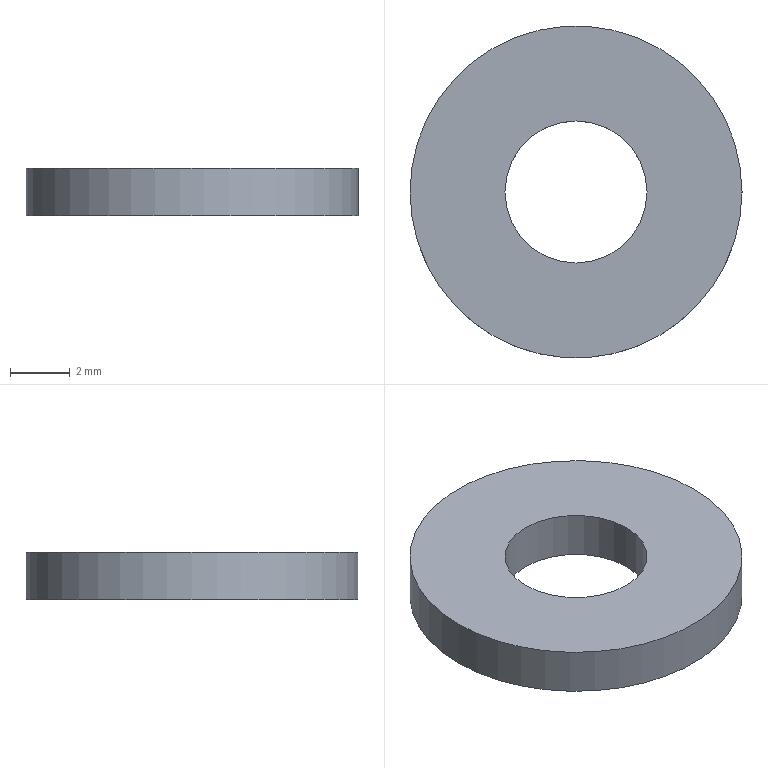Part | NX | features solid 2 | 1 solid | 4 faces | box 11.125 x 11.125 x 1.6 mm | volume 127.031 mm3 | cylinder 2 | plane 2 | commonest cylinder face diameters 4.763 x1 11.125 x1
STEP:
#1=CARTESIAN_POINT('',(5.563,0.,1.6));
#2=VERTEX_POINT('',#1);
#3=CARTESIAN_POINT('',(0.,0.,1.6));
#4=DIRECTION('',(0.,0.,1.));
#5=DIRECTION('',(1.,0.,0.));
#6=AXIS2_PLACEMENT_3D('',#3,#4,#5);
#7=CIRCLE('',#6,5.563);
#8=EDGE_CURVE('',#2,#2,#7,.T.);
#9=ORIENTED_EDGE('',*,*,#8,.F.);
#10=EDGE_LOOP('',(#9));
#11=FACE_BOUND('',#10,.T.);
#12=CARTESIAN_POINT('',(5.563,0.,0.));
#13=VERTEX_POINT('',#12);
#14=CARTESIAN_POINT('',(0.,0.,0.));
#15=DIRECTION('',(0.,0.,1.));
#16=DIRECTION('',(1.,0.,0.));
#17=AXIS2_PLACEMENT_3D('',#14,#15,#16);
#18=CIRCLE('',#17,5.563);
#19=EDGE_CURVE('',#13,#13,#18,.T.);
#20=ORIENTED_EDGE('',*,*,#19,.T.);
#21=EDGE_LOOP('',(#20));
#22=FACE_BOUND('',#21,.T.);
#23=CARTESIAN_POINT('',(0.,0.,1.6));
#24=DIRECTION('',(0.,0.,-1.));
#25=DIRECTION('',(-1.,0.,0.));
#26=AXIS2_PLACEMENT_3D('',#23,#24,#25);
#27=CYLINDRICAL_SURFACE('',#26,5.563);
#28=ADVANCED_FACE('',(#11,#22),#27,.T.);
#29=CARTESIAN_POINT('',(2.381,0.,1.6));
#30=VERTEX_POINT('',#29);
#31=CARTESIAN_POINT('',(0.,0.,1.6));
#32=DIRECTION('',(0.,0.,1.));
#33=DIRECTION('',(1.,0.,0.));
#34=AXIS2_PLACEMENT_3D('',#31,#32,#33);
#35=CIRCLE('',#34,2.381);
#36=EDGE_CURVE('',#30,#30,#35,.T.);
#37=ORIENTED_EDGE('',*,*,#36,.T.);
#38=EDGE_LOOP('',(#37));
#39=FACE_BOUND('',#38,.T.);
#40=CARTESIAN_POINT('',(2.381,0.,0.));
#41=VERTEX_POINT('',#40);
#42=CARTESIAN_POINT('',(0.,0.,0.));
#43=DIRECTION('',(0.,0.,1.));
#44=DIRECTION('',(1.,0.,0.));
#45=AXIS2_PLACEMENT_3D('',#42,#43,#44);
#46=CIRCLE('',#45,2.381);
#47=EDGE_CURVE('',#41,#41,#46,.T.);
#48=ORIENTED_EDGE('',*,*,#47,.F.);
#49=EDGE_LOOP('',(#48));
#50=FACE_BOUND('',#49,.T.);
#51=CARTESIAN_POINT('',(0.,0.,1.6));
#52=DIRECTION('',(0.,0.,-1.));
#53=DIRECTION('',(-1.,0.,0.));
#54=AXIS2_PLACEMENT_3D('',#51,#52,#53);
#55=CYLINDRICAL_SURFACE('',#54,2.381);
#56=ADVANCED_FACE('',(#39,#50),#55,.F.);
#57=ORIENTED_EDGE('',*,*,#8,.T.);
#58=EDGE_LOOP('',(#57));
#59=FACE_BOUND('',#58,.T.);
#60=ORIENTED_EDGE('',*,*,#36,.F.);
#61=EDGE_LOOP('',(#60));
#62=FACE_BOUND('',#61,.T.);
#63=CARTESIAN_POINT('',(0.,0.,1.6));
#64=DIRECTION('',(0.,0.,1.));
#65=DIRECTION('',(1.,0.,0.));
#66=AXIS2_PLACEMENT_3D('',#63,#64,#65);
#67=PLANE('',#66);
#68=ADVANCED_FACE('',(#59,#62),#67,.T.);
#69=ORIENTED_EDGE('',*,*,#19,.F.);
#70=EDGE_LOOP('',(#69));
#71=FACE_BOUND('',#70,.T.);
#72=ORIENTED_EDGE('',*,*,#47,.T.);
#73=EDGE_LOOP('',(#72));
#74=FACE_BOUND('',#73,.T.);
#75=CARTESIAN_POINT('',(0.,0.,0.));
#76=DIRECTION('',(0.,0.,1.));
#77=DIRECTION('',(1.,0.,0.));
#78=AXIS2_PLACEMENT_3D('',#75,#76,#77);
#79=PLANE('',#78);
#80=ADVANCED_FACE('',(#71,#74),#79,.F.);
#81=CLOSED_SHELL('',(#28,#56,#68,#80));
#82=MANIFOLD_SOLID_BREP('',#81);
#83=(LENGTH_UNIT()NAMED_UNIT(*)SI_UNIT(.MILLI.,.METRE.));
#84=UNCERTAINTY_MEASURE_WITH_UNIT(LENGTH_MEASURE(0.00001),#83,'','');
#85=(NAMED_UNIT(*)PLANE_ANGLE_UNIT()SI_UNIT($,.RADIAN.));
#86=(NAMED_UNIT(*)SI_UNIT($,.STERADIAN.)SOLID_ANGLE_UNIT());
#87=(GEOMETRIC_REPRESENTATION_CONTEXT(3)GLOBAL_UNCERTAINTY_ASSIGNED_CONTEXT((#84))GLOBAL_UNIT_ASSIGNED_CONTEXT((#83,#85,#86))REPRESENTATION_CONTEXT('',''));
#88=ADVANCED_BREP_SHAPE_REPRESENTATION('',(#82),#87);